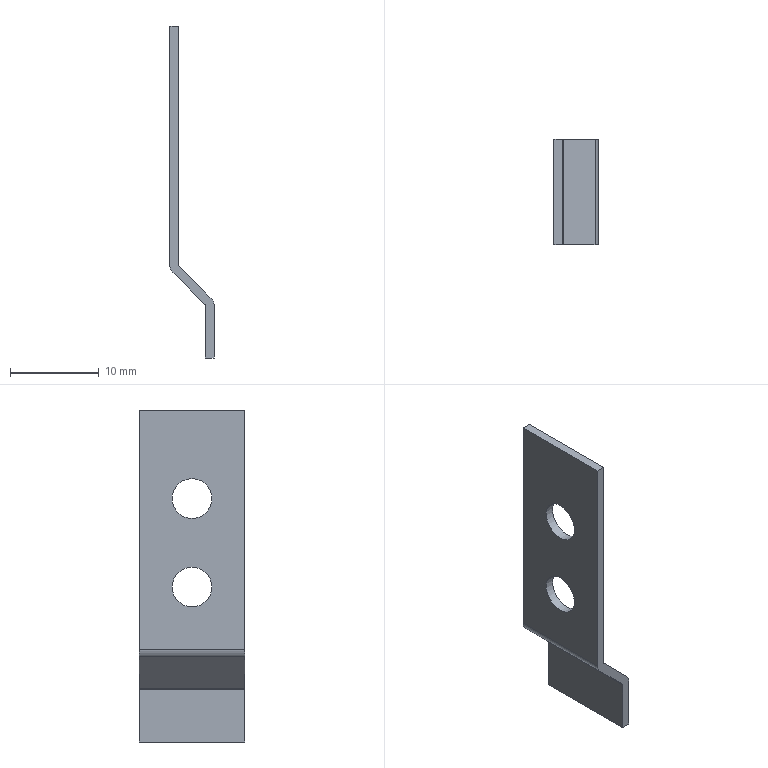Part | STEP file | 1 solid | 16 faces | box 5 x 11.9 x 37.5 mm | volume 433.441 mm3 | plane 10 | cylinder 6 | commonest cylinder face diameters 0.4 x2 2.4 x2 4.5 x2
STEP:
#1=CARTESIAN_POINT('',(0.,0.,0.));
#2=DIRECTION('',(0.,0.,1.));
#3=DIRECTION('',(1.,0.,0.));
#4=AXIS2_PLACEMENT_3D('',#1,#2,#3);
#5=CARTESIAN_POINT('',(0.,0.,-17.75));
#6=VERTEX_POINT('',#5);
#7=CARTESIAN_POINT('',(0.,0.,-20.));
#8=DIRECTION('',(1.,0.,0.));
#9=DIRECTION('',(0.,0.,1.));
#10=AXIS2_PLACEMENT_3D('',#7,#8,#9);
#11=CIRCLE('',#10,2.25);
#12=CARTESIAN_POINT('',(0.,5.95,0.));
#13=DIRECTION('',(-1.,0.,0.));
#14=DIRECTION('',(0.,0.,1.));
#15=AXIS2_PLACEMENT_3D('',#12,#13,#14);
#16=PLANE('',#15);
#17=CARTESIAN_POINT('',(-17.75,-5.95));
#18=CARTESIAN_POINT('',(-17.75,-9.847));
#19=CARTESIAN_POINT('',(-21.125,-7.899));
#20=CARTESIAN_POINT('',(-24.5,-5.95));
#21=CARTESIAN_POINT('',(-21.125,-4.001));
#22=CARTESIAN_POINT('',(-17.75,-2.053));
#23=CARTESIAN_POINT('',(-17.75,-5.95));
#24=(BOUNDED_CURVE()B_SPLINE_CURVE(2,(#17,#18,#19,#20,#21,#22,#23),.UNSPECIFIED.,.T.,.F.)B_SPLINE_CURVE_WITH_KNOTS((1,2,2,2,2,1),(-2.094,0.,2.094,4.189,6.283,8.378),.UNSPECIFIED.)CURVE()GEOMETRIC_REPRESENTATION_ITEM()RATIONAL_B_SPLINE_CURVE((1.,0.5,1.,0.5,1.,0.5,1.))REPRESENTATION_ITEM(''));
#25=(GEOMETRIC_REPRESENTATION_CONTEXT(2)PARAMETRIC_REPRESENTATION_CONTEXT()REPRESENTATION_CONTEXT('',''));
#26=DEFINITIONAL_REPRESENTATION('',(#24),#25);
#27=PCURVE('',#16,#26);
#28=CARTESIAN_POINT('',(0.,0.,-20.));
#29=DIRECTION('',(-1.,0.,0.));
#30=DIRECTION('',(0.,0.,1.));
#31=AXIS2_PLACEMENT_3D('',#28,#29,#30);
#32=CYLINDRICAL_SURFACE('',#31,2.25);
#33=CARTESIAN_POINT('',(6.283,0.));
#34=DIRECTION('',(-1.,0.));
#35=VECTOR('',#34,1.);
#36=LINE('',#33,#35);
#37=(GEOMETRIC_REPRESENTATION_CONTEXT(2)PARAMETRIC_REPRESENTATION_CONTEXT()REPRESENTATION_CONTEXT('',''));
#38=DEFINITIONAL_REPRESENTATION('',(#36),#37);
#39=PCURVE('',#32,#38);
#40=SURFACE_CURVE('',#11,(#27,#39),.PCURVE_S1.);
#41=EDGE_CURVE('',#6,#6,#40,.T.);
#42=ORIENTED_EDGE('',*,*,#41,.T.);
#43=EDGE_LOOP('',(#42));
#44=FACE_BOUND('',#43,.T.);
#45=CARTESIAN_POINT('',(0.,0.,-7.75));
#46=VERTEX_POINT('',#45);
#47=CARTESIAN_POINT('',(0.,0.,-10.));
#48=DIRECTION('',(1.,0.,0.));
#49=DIRECTION('',(0.,0.,1.));
#50=AXIS2_PLACEMENT_3D('',#47,#48,#49);
#51=CIRCLE('',#50,2.25);
#52=CARTESIAN_POINT('',(-7.75,-5.95));
#53=CARTESIAN_POINT('',(-7.75,-9.847));
#54=CARTESIAN_POINT('',(-11.125,-7.899));
#55=CARTESIAN_POINT('',(-14.5,-5.95));
#56=CARTESIAN_POINT('',(-11.125,-4.001));
#57=CARTESIAN_POINT('',(-7.75,-2.053));
#58=CARTESIAN_POINT('',(-7.75,-5.95));
#59=(BOUNDED_CURVE()B_SPLINE_CURVE(2,(#52,#53,#54,#55,#56,#57,#58),.UNSPECIFIED.,.T.,.F.)B_SPLINE_CURVE_WITH_KNOTS((1,2,2,2,2,1),(-2.094,0.,2.094,4.189,6.283,8.378),.UNSPECIFIED.)CURVE()GEOMETRIC_REPRESENTATION_ITEM()RATIONAL_B_SPLINE_CURVE((1.,0.5,1.,0.5,1.,0.5,1.))REPRESENTATION_ITEM(''));
#60=(GEOMETRIC_REPRESENTATION_CONTEXT(2)PARAMETRIC_REPRESENTATION_CONTEXT()REPRESENTATION_CONTEXT('',''));
#61=DEFINITIONAL_REPRESENTATION('',(#59),#60);
#62=PCURVE('',#16,#61);
#63=CARTESIAN_POINT('',(0.,0.,-10.));
#64=DIRECTION('',(-1.,0.,0.));
#65=DIRECTION('',(0.,0.,1.));
#66=AXIS2_PLACEMENT_3D('',#63,#64,#65);
#67=CYLINDRICAL_SURFACE('',#66,2.25);
#68=CARTESIAN_POINT('',(6.283,0.));
#69=DIRECTION('',(-1.,0.));
#70=VECTOR('',#69,1.);
#71=LINE('',#68,#70);
#72=(GEOMETRIC_REPRESENTATION_CONTEXT(2)PARAMETRIC_REPRESENTATION_CONTEXT()REPRESENTATION_CONTEXT('',''));
#73=DEFINITIONAL_REPRESENTATION('',(#71),#72);
#74=PCURVE('',#67,#73);
#75=SURFACE_CURVE('',#51,(#62,#74),.PCURVE_S1.);
#76=EDGE_CURVE('',#46,#46,#75,.T.);
#77=ORIENTED_EDGE('',*,*,#76,.T.);
#78=EDGE_LOOP('',(#77));
#79=FACE_BOUND('',#78,.T.);
#80=CARTESIAN_POINT('',(0.,5.95,0.));
#81=VERTEX_POINT('',#80);
#82=CARTESIAN_POINT('',(0.,5.95,-27.003));
#83=VERTEX_POINT('',#82);
#84=CARTESIAN_POINT('',(0.,5.95,0.));
#85=DIRECTION('',(0.,0.,-1.));
#86=VECTOR('',#85,1.);
#87=LINE('',#84,#86);
#88=CARTESIAN_POINT('',(0.,0.));
#89=DIRECTION('',(-1.,0.));
#90=VECTOR('',#89,1.);
#91=LINE('',#88,#90);
#92=(GEOMETRIC_REPRESENTATION_CONTEXT(2)PARAMETRIC_REPRESENTATION_CONTEXT()REPRESENTATION_CONTEXT('',''));
#93=DEFINITIONAL_REPRESENTATION('',(#91),#92);
#94=PCURVE('',#16,#93);
#95=CARTESIAN_POINT('',(3.8,5.95,-31.583));
#96=DIRECTION('',(0.,-1.,0.));
#97=DIRECTION('',(0.,0.,-1.));
#98=AXIS2_PLACEMENT_3D('',#95,#96,#97);
#99=PLANE('',#98);
#100=CARTESIAN_POINT('',(-31.583,-3.8));
#101=DIRECTION('',(1.,0.));
#102=VECTOR('',#101,1.);
#103=LINE('',#100,#102);
#104=(GEOMETRIC_REPRESENTATION_CONTEXT(2)PARAMETRIC_REPRESENTATION_CONTEXT()REPRESENTATION_CONTEXT('',''));
#105=DEFINITIONAL_REPRESENTATION('',(#103),#104);
#106=PCURVE('',#99,#105);
#107=SURFACE_CURVE('',#87,(#94,#106),.PCURVE_S1.);
#108=EDGE_CURVE('',#81,#83,#107,.T.);
#109=ORIENTED_EDGE('',*,*,#108,.T.);
#110=CARTESIAN_POINT('',(0.,-5.95,-27.003));
#111=VERTEX_POINT('',#110);
#112=CARTESIAN_POINT('',(0.,5.95,-27.003));
#113=DIRECTION('',(0.,-1.,0.));
#114=VECTOR('',#113,1.);
#115=LINE('',#112,#114);
#116=CARTESIAN_POINT('',(-27.003,0.));
#117=DIRECTION('',(0.,-1.));
#118=VECTOR('',#117,1.);
#119=LINE('',#116,#118);
#120=(GEOMETRIC_REPRESENTATION_CONTEXT(2)PARAMETRIC_REPRESENTATION_CONTEXT()REPRESENTATION_CONTEXT('',''));
#121=DEFINITIONAL_REPRESENTATION('',(#119),#120);
#122=PCURVE('',#16,#121);
#123=CARTESIAN_POINT('',(1.2,5.95,-27.003));
#124=DIRECTION('',(0.,-1.,0.));
#125=DIRECTION('',(0.,0.,-1.));
#126=AXIS2_PLACEMENT_3D('',#123,#124,#125);
#127=CYLINDRICAL_SURFACE('',#126,1.2);
#128=CARTESIAN_POINT('',(4.712,0.));
#129=DIRECTION('',(0.,1.));
#130=VECTOR('',#129,1.);
#131=LINE('',#128,#130);
#132=(GEOMETRIC_REPRESENTATION_CONTEXT(2)PARAMETRIC_REPRESENTATION_CONTEXT()REPRESENTATION_CONTEXT('',''));
#133=DEFINITIONAL_REPRESENTATION('',(#131),#132);
#134=PCURVE('',#127,#133);
#135=SURFACE_CURVE('',#115,(#122,#134),.PCURVE_S1.);
#136=EDGE_CURVE('',#83,#111,#135,.T.);
#137=ORIENTED_EDGE('',*,*,#136,.T.);
#138=CARTESIAN_POINT('',(0.,-5.95,0.));
#139=VERTEX_POINT('',#138);
#140=CARTESIAN_POINT('',(0.,-5.95,0.));
#141=DIRECTION('',(0.,0.,1.));
#142=VECTOR('',#141,1.);
#143=LINE('',#140,#142);
#144=CARTESIAN_POINT('',(0.,-11.9));
#145=DIRECTION('',(1.,0.));
#146=VECTOR('',#145,1.);
#147=LINE('',#144,#146);
#148=(GEOMETRIC_REPRESENTATION_CONTEXT(2)PARAMETRIC_REPRESENTATION_CONTEXT()REPRESENTATION_CONTEXT('',''));
#149=DEFINITIONAL_REPRESENTATION('',(#147),#148);
#150=PCURVE('',#16,#149);
#151=CARTESIAN_POINT('',(1.059,-5.95,-27.144));
#152=DIRECTION('',(0.,-1.,0.));
#153=DIRECTION('',(0.,0.,-1.));
#154=AXIS2_PLACEMENT_3D('',#151,#152,#153);
#155=PLANE('',#154);
#156=CARTESIAN_POINT('',(-27.144,-1.059));
#157=DIRECTION('',(-1.,0.));
#158=VECTOR('',#157,1.);
#159=LINE('',#156,#158);
#160=(GEOMETRIC_REPRESENTATION_CONTEXT(2)PARAMETRIC_REPRESENTATION_CONTEXT()REPRESENTATION_CONTEXT('',''));
#161=DEFINITIONAL_REPRESENTATION('',(#159),#160);
#162=PCURVE('',#155,#161);
#163=SURFACE_CURVE('',#143,(#150,#162),.PCURVE_S1.);
#164=EDGE_CURVE('',#111,#139,#163,.T.);
#165=ORIENTED_EDGE('',*,*,#164,.T.);
#166=CARTESIAN_POINT('',(0.,5.95,0.));
#167=DIRECTION('',(0.,1.,0.));
#168=VECTOR('',#167,1.);
#169=LINE('',#166,#168);
#170=CARTESIAN_POINT('',(0.,0.));
#171=DIRECTION('',(0.,1.));
#172=VECTOR('',#171,1.);
#173=LINE('',#170,#172);
#174=(GEOMETRIC_REPRESENTATION_CONTEXT(2)PARAMETRIC_REPRESENTATION_CONTEXT()REPRESENTATION_CONTEXT('',''));
#175=DEFINITIONAL_REPRESENTATION('',(#173),#174);
#176=PCURVE('',#16,#175);
#177=CARTESIAN_POINT('',(1.,5.95,0.));
#178=DIRECTION('',(0.,0.,1.));
#179=DIRECTION('',(1.,0.,0.));
#180=AXIS2_PLACEMENT_3D('',#177,#178,#179);
#181=PLANE('',#180);
#182=CARTESIAN_POINT('',(-1.,0.));
#183=DIRECTION('',(0.,1.));
#184=VECTOR('',#183,1.);
#185=LINE('',#182,#184);
#186=(GEOMETRIC_REPRESENTATION_CONTEXT(2)PARAMETRIC_REPRESENTATION_CONTEXT()REPRESENTATION_CONTEXT('',''));
#187=DEFINITIONAL_REPRESENTATION('',(#185),#186);
#188=PCURVE('',#181,#187);
#189=SURFACE_CURVE('',#169,(#176,#188),.PCURVE_S1.);
#190=EDGE_CURVE('',#139,#81,#189,.T.);
#191=ORIENTED_EDGE('',*,*,#190,.T.);
#192=EDGE_LOOP('',(#109,#137,#165,#191));
#193=FACE_BOUND('',#192,.T.);
#194=ADVANCED_FACE('',(#44,#79,#193),#16,.T.);
#195=ORIENTED_EDGE('',*,*,#41,.T.);
#196=CARTESIAN_POINT('',(1.,0.,-17.75));
#197=VERTEX_POINT('',#196);
#198=CARTESIAN_POINT('',(1.,0.,-17.75));
#199=CARTESIAN_POINT('',(0.,0.,-17.75));
#200=B_SPLINE_CURVE_WITH_KNOTS('',1,(#198,#199),.UNSPECIFIED.,.F.,.F.,(2,2),(-1.,0.),.PIECEWISE_BEZIER_KNOTS.);
#201=CARTESIAN_POINT('',(0.,0.));
#202=DIRECTION('',(0.,1.));
#203=VECTOR('',#202,1.);
#204=LINE('',#201,#203);
#205=(GEOMETRIC_REPRESENTATION_CONTEXT(2)PARAMETRIC_REPRESENTATION_CONTEXT()REPRESENTATION_CONTEXT('',''));
#206=DEFINITIONAL_REPRESENTATION('',(#204),#205);
#207=PCURVE('',#32,#206);
#208=CARTESIAN_POINT('',(6.283,0.));
#209=DIRECTION('',(0.,1.));
#210=VECTOR('',#209,1.);
#211=LINE('',#208,#210);
#212=(GEOMETRIC_REPRESENTATION_CONTEXT(2)PARAMETRIC_REPRESENTATION_CONTEXT()REPRESENTATION_CONTEXT('',''));
#213=DEFINITIONAL_REPRESENTATION('',(#211),#212);
#214=PCURVE('',#32,#213);
#215=SEAM_CURVE('',#200,(#207,#214),.PCURVE_S1.);
#216=EDGE_CURVE('',#197,#6,#215,.T.);
#217=ORIENTED_EDGE('',*,*,#216,.F.);
#218=CARTESIAN_POINT('',(1.,0.,-20.));
#219=DIRECTION('',(-1.,0.,0.));
#220=DIRECTION('',(0.,0.,1.));
#221=AXIS2_PLACEMENT_3D('',#218,#219,#220);
#222=CIRCLE('',#221,2.25);
#223=CARTESIAN_POINT('',(0.,-1.));
#224=DIRECTION('',(1.,0.));
#225=VECTOR('',#224,1.);
#226=LINE('',#223,#225);
#227=(GEOMETRIC_REPRESENTATION_CONTEXT(2)PARAMETRIC_REPRESENTATION_CONTEXT()REPRESENTATION_CONTEXT('',''));
#228=DEFINITIONAL_REPRESENTATION('',(#226),#227);
#229=PCURVE('',#32,#228);
#230=CARTESIAN_POINT('',(1.,5.95,0.));
#231=DIRECTION('',(-1.,0.,0.));
#232=DIRECTION('',(0.,0.,1.));
#233=AXIS2_PLACEMENT_3D('',#230,#231,#232);
#234=PLANE('',#233);
#235=CARTESIAN_POINT('',(-20.,-5.95));
#236=DIRECTION('',(1.,0.));
#237=AXIS2_PLACEMENT_2D('',#235,#236);
#238=CIRCLE('',#237,2.25);
#239=(GEOMETRIC_REPRESENTATION_CONTEXT(2)PARAMETRIC_REPRESENTATION_CONTEXT()REPRESENTATION_CONTEXT('',''));
#240=DEFINITIONAL_REPRESENTATION('',(#238),#239);
#241=PCURVE('',#234,#240);
#242=SURFACE_CURVE('',#222,(#229,#241),.PCURVE_S1.);
#243=EDGE_CURVE('',#197,#197,#242,.T.);
#244=ORIENTED_EDGE('',*,*,#243,.T.);
#245=ORIENTED_EDGE('',*,*,#216,.T.);
#246=EDGE_LOOP('',(#195,#217,#244,#245));
#247=FACE_BOUND('',#246,.F.);
#248=ADVANCED_FACE('',(#247),#32,.F.);
#249=ORIENTED_EDGE('',*,*,#76,.T.);
#250=CARTESIAN_POINT('',(1.,0.,-7.75));
#251=VERTEX_POINT('',#250);
#252=CARTESIAN_POINT('',(1.,0.,-7.75));
#253=CARTESIAN_POINT('',(0.,0.,-7.75));
#254=B_SPLINE_CURVE_WITH_KNOTS('',1,(#252,#253),.UNSPECIFIED.,.F.,.F.,(2,2),(-1.,0.),.PIECEWISE_BEZIER_KNOTS.);
#255=CARTESIAN_POINT('',(0.,0.));
#256=DIRECTION('',(0.,1.));
#257=VECTOR('',#256,1.);
#258=LINE('',#255,#257);
#259=(GEOMETRIC_REPRESENTATION_CONTEXT(2)PARAMETRIC_REPRESENTATION_CONTEXT()REPRESENTATION_CONTEXT('',''));
#260=DEFINITIONAL_REPRESENTATION('',(#258),#259);
#261=PCURVE('',#67,#260);
#262=CARTESIAN_POINT('',(6.283,0.));
#263=DIRECTION('',(0.,1.));
#264=VECTOR('',#263,1.);
#265=LINE('',#262,#264);
#266=(GEOMETRIC_REPRESENTATION_CONTEXT(2)PARAMETRIC_REPRESENTATION_CONTEXT()REPRESENTATION_CONTEXT('',''));
#267=DEFINITIONAL_REPRESENTATION('',(#265),#266);
#268=PCURVE('',#67,#267);
#269=SEAM_CURVE('',#254,(#261,#268),.PCURVE_S1.);
#270=EDGE_CURVE('',#251,#46,#269,.T.);
#271=ORIENTED_EDGE('',*,*,#270,.F.);
#272=CARTESIAN_POINT('',(1.,0.,-10.));
#273=DIRECTION('',(-1.,0.,0.));
#274=DIRECTION('',(0.,0.,1.));
#275=AXIS2_PLACEMENT_3D('',#272,#273,#274);
#276=CIRCLE('',#275,2.25);
#277=CARTESIAN_POINT('',(0.,-1.));
#278=DIRECTION('',(1.,0.));
#279=VECTOR('',#278,1.);
#280=LINE('',#277,#279);
#281=(GEOMETRIC_REPRESENTATION_CONTEXT(2)PARAMETRIC_REPRESENTATION_CONTEXT()REPRESENTATION_CONTEXT('',''));
#282=DEFINITIONAL_REPRESENTATION('',(#280),#281);
#283=PCURVE('',#67,#282);
#284=CARTESIAN_POINT('',(-10.,-5.95));
#285=DIRECTION('',(1.,0.));
#286=AXIS2_PLACEMENT_2D('',#284,#285);
#287=CIRCLE('',#286,2.25);
#288=(GEOMETRIC_REPRESENTATION_CONTEXT(2)PARAMETRIC_REPRESENTATION_CONTEXT()REPRESENTATION_CONTEXT('',''));
#289=DEFINITIONAL_REPRESENTATION('',(#287),#288);
#290=PCURVE('',#234,#289);
#291=SURFACE_CURVE('',#276,(#283,#290),.PCURVE_S1.);
#292=EDGE_CURVE('',#251,#251,#291,.T.);
#293=ORIENTED_EDGE('',*,*,#292,.T.);
#294=ORIENTED_EDGE('',*,*,#270,.T.);
#295=EDGE_LOOP('',(#249,#271,#293,#294));
#296=FACE_BOUND('',#295,.F.);
#297=ADVANCED_FACE('',(#296),#67,.F.);
#298=CARTESIAN_POINT('',(0.3515,5.95,-27.851));
#299=VERTEX_POINT('',#298);
#300=CARTESIAN_POINT('',(1.2,5.95,-27.003));
#301=DIRECTION('',(0.,-1.,0.));
#302=DIRECTION('',(0.,0.,-1.));
#303=AXIS2_PLACEMENT_3D('',#300,#301,#302);
#304=CIRCLE('',#303,1.2);
#305=CARTESIAN_POINT('',(0.,0.));
#306=DIRECTION('',(1.,0.));
#307=VECTOR('',#306,1.);
#308=LINE('',#305,#307);
#309=(GEOMETRIC_REPRESENTATION_CONTEXT(2)PARAMETRIC_REPRESENTATION_CONTEXT()REPRESENTATION_CONTEXT('',''));
#310=DEFINITIONAL_REPRESENTATION('',(#308),#309);
#311=PCURVE('',#127,#310);
#312=CARTESIAN_POINT('',(-4.58,-2.6));
#313=DIRECTION('',(1.,0.));
#314=AXIS2_PLACEMENT_2D('',#312,#313);
#315=CIRCLE('',#314,1.2);
#316=(GEOMETRIC_REPRESENTATION_CONTEXT(2)PARAMETRIC_REPRESENTATION_CONTEXT()REPRESENTATION_CONTEXT('',''));
#317=DEFINITIONAL_REPRESENTATION('',(#315),#316);
#318=PCURVE('',#99,#317);
#319=SURFACE_CURVE('',#304,(#311,#318),.PCURVE_S1.);
#320=EDGE_CURVE('',#83,#299,#319,.T.);
#321=ORIENTED_EDGE('',*,*,#320,.T.);
#322=CARTESIAN_POINT('',(0.3515,-5.95,-27.851));
#323=VERTEX_POINT('',#322);
#324=CARTESIAN_POINT('',(0.3515,5.95,-27.851));
#325=DIRECTION('',(0.,-1.,0.));
#326=VECTOR('',#325,1.);
#327=LINE('',#324,#326);
#328=CARTESIAN_POINT('',(5.498,0.));
#329=DIRECTION('',(0.,1.));
#330=VECTOR('',#329,1.);
#331=LINE('',#328,#330);
#332=(GEOMETRIC_REPRESENTATION_CONTEXT(2)PARAMETRIC_REPRESENTATION_CONTEXT()REPRESENTATION_CONTEXT('',''));
#333=DEFINITIONAL_REPRESENTATION('',(#331),#332);
#334=PCURVE('',#127,#333);
#335=CARTESIAN_POINT('',(0.,5.95,-27.5));
#336=DIRECTION('',(-0.7071,0.,-0.7071));
#337=DIRECTION('',(-0.7071,0.,0.7071));
#338=AXIS2_PLACEMENT_3D('',#335,#336,#337);
#339=PLANE('',#338);
#340=CARTESIAN_POINT('',(-0.4971,0.));
#341=DIRECTION('',(0.,-1.));
#342=VECTOR('',#341,1.);
#343=LINE('',#340,#342);
#344=(GEOMETRIC_REPRESENTATION_CONTEXT(2)PARAMETRIC_REPRESENTATION_CONTEXT()REPRESENTATION_CONTEXT('',''));
#345=DEFINITIONAL_REPRESENTATION('',(#343),#344);
#346=PCURVE('',#339,#345);
#347=SURFACE_CURVE('',#327,(#334,#346),.PCURVE_S1.);
#348=EDGE_CURVE('',#299,#323,#347,.T.);
#349=ORIENTED_EDGE('',*,*,#348,.T.);
#350=CARTESIAN_POINT('',(1.2,-5.95,-27.003));
#351=DIRECTION('',(0.,1.,0.));
#352=DIRECTION('',(0.,0.,-1.));
#353=AXIS2_PLACEMENT_3D('',#350,#351,#352);
#354=CIRCLE('',#353,1.2);
#355=CARTESIAN_POINT('',(6.283,11.9));
#356=DIRECTION('',(-1.,0.));
#357=VECTOR('',#356,1.);
#358=LINE('',#355,#357);
#359=(GEOMETRIC_REPRESENTATION_CONTEXT(2)PARAMETRIC_REPRESENTATION_CONTEXT()REPRESENTATION_CONTEXT('',''));
#360=DEFINITIONAL_REPRESENTATION('',(#358),#359);
#361=PCURVE('',#127,#360);
#362=CARTESIAN_POINT('',(1.059,0.1414));
#363=CARTESIAN_POINT('',(1.059,-1.937));
#364=CARTESIAN_POINT('',(-0.7414,-0.8978));
#365=CARTESIAN_POINT('',(-2.541,0.1414));
#366=CARTESIAN_POINT('',(-0.7414,1.181));
#367=CARTESIAN_POINT('',(1.059,2.22));
#368=CARTESIAN_POINT('',(1.059,0.1414));
#369=(BOUNDED_CURVE()B_SPLINE_CURVE(2,(#362,#363,#364,#365,#366,#367,#368),.UNSPECIFIED.,.T.,.F.)B_SPLINE_CURVE_WITH_KNOTS((1,2,2,2,2,1),(-2.094,0.,2.094,4.189,6.283,8.378),.UNSPECIFIED.)CURVE()GEOMETRIC_REPRESENTATION_ITEM()RATIONAL_B_SPLINE_CURVE((1.,0.5,1.,0.5,1.,0.5,1.))REPRESENTATION_ITEM(''));
#370=(GEOMETRIC_REPRESENTATION_CONTEXT(2)PARAMETRIC_REPRESENTATION_CONTEXT()REPRESENTATION_CONTEXT('',''));
#371=DEFINITIONAL_REPRESENTATION('',(#369),#370);
#372=PCURVE('',#155,#371);
#373=SURFACE_CURVE('',#354,(#361,#372),.PCURVE_S1.);
#374=EDGE_CURVE('',#323,#111,#373,.T.);
#375=ORIENTED_EDGE('',*,*,#374,.T.);
#376=ORIENTED_EDGE('',*,*,#136,.F.);
#377=EDGE_LOOP('',(#321,#349,#375,#376));
#378=FACE_BOUND('',#377,.T.);
#379=ADVANCED_FACE('',(#378),#127,.T.);
#380=CARTESIAN_POINT('',(1.,5.95,-27.003));
#381=VERTEX_POINT('',#380);
#382=CARTESIAN_POINT('',(1.,5.95,0.));
#383=VERTEX_POINT('',#382);
#384=CARTESIAN_POINT('',(1.,5.95,-31.583));
#385=DIRECTION('',(0.,0.,1.));
#386=VECTOR('',#385,1.);
#387=LINE('',#384,#386);
#388=CARTESIAN_POINT('',(0.,-2.8));
#389=DIRECTION('',(-1.,0.));
#390=VECTOR('',#389,1.);
#391=LINE('',#388,#390);
#392=(GEOMETRIC_REPRESENTATION_CONTEXT(2)PARAMETRIC_REPRESENTATION_CONTEXT()REPRESENTATION_CONTEXT('',''));
#393=DEFINITIONAL_REPRESENTATION('',(#391),#392);
#394=PCURVE('',#99,#393);
#395=CARTESIAN_POINT('',(-31.583,0.));
#396=DIRECTION('',(1.,0.));
#397=VECTOR('',#396,1.);
#398=LINE('',#395,#397);
#399=(GEOMETRIC_REPRESENTATION_CONTEXT(2)PARAMETRIC_REPRESENTATION_CONTEXT()REPRESENTATION_CONTEXT('',''));
#400=DEFINITIONAL_REPRESENTATION('',(#398),#399);
#401=PCURVE('',#234,#400);
#402=SURFACE_CURVE('',#387,(#394,#401),.PCURVE_S1.);
#403=EDGE_CURVE('',#381,#383,#402,.T.);
#404=ORIENTED_EDGE('',*,*,#403,.F.);
#405=CARTESIAN_POINT('',(1.059,5.95,-27.144));
#406=VERTEX_POINT('',#405);
#407=CARTESIAN_POINT('',(1.2,5.95,-27.003));
#408=DIRECTION('',(0.,-1.,0.));
#409=DIRECTION('',(0.,0.,-1.));
#410=AXIS2_PLACEMENT_3D('',#407,#408,#409);
#411=CIRCLE('',#410,0.2);
#412=CARTESIAN_POINT('',(-4.58,-2.6));
#413=DIRECTION('',(1.,0.));
#414=AXIS2_PLACEMENT_2D('',#412,#413);
#415=CIRCLE('',#414,0.2);
#416=(GEOMETRIC_REPRESENTATION_CONTEXT(2)PARAMETRIC_REPRESENTATION_CONTEXT()REPRESENTATION_CONTEXT('',''));
#417=DEFINITIONAL_REPRESENTATION('',(#415),#416);
#418=PCURVE('',#99,#417);
#419=CARTESIAN_POINT('',(1.2,5.95,-27.003));
#420=DIRECTION('',(0.,-1.,0.));
#421=DIRECTION('',(0.,0.,-1.));
#422=AXIS2_PLACEMENT_3D('',#419,#420,#421);
#423=CYLINDRICAL_SURFACE('',#422,0.2);
#424=CARTESIAN_POINT('',(0.,0.));
#425=DIRECTION('',(1.,0.));
#426=VECTOR('',#425,1.);
#427=LINE('',#424,#426);
#428=(GEOMETRIC_REPRESENTATION_CONTEXT(2)PARAMETRIC_REPRESENTATION_CONTEXT()REPRESENTATION_CONTEXT('',''));
#429=DEFINITIONAL_REPRESENTATION('',(#427),#428);
#430=PCURVE('',#423,#429);
#431=SURFACE_CURVE('',#411,(#418,#430),.PCURVE_S1.);
#432=EDGE_CURVE('',#381,#406,#431,.T.);
#433=ORIENTED_EDGE('',*,*,#432,.T.);
#434=CARTESIAN_POINT('',(4.649,5.95,-30.734));
#435=VERTEX_POINT('',#434);
#436=CARTESIAN_POINT('',(1.059,5.95,-27.144));
#437=DIRECTION('',(0.7071,0.,-0.7071));
#438=VECTOR('',#437,1.);
#439=LINE('',#436,#438);
#440=CARTESIAN_POINT('',(-4.438,-2.741));
#441=DIRECTION('',(0.7071,0.7071));
#442=VECTOR('',#441,1.);
#443=LINE('',#440,#442);
#444=(GEOMETRIC_REPRESENTATION_CONTEXT(2)PARAMETRIC_REPRESENTATION_CONTEXT()REPRESENTATION_CONTEXT('',''));
#445=DEFINITIONAL_REPRESENTATION('',(#443),#444);
#446=PCURVE('',#99,#445);
#447=CARTESIAN_POINT('',(0.7071,5.95,-26.793));
#448=DIRECTION('',(-0.7071,0.,-0.7071));
#449=DIRECTION('',(-0.7071,0.,0.7071));
#450=AXIS2_PLACEMENT_3D('',#447,#448,#449);
#451=PLANE('',#450);
#452=CARTESIAN_POINT('',(-0.4971,0.));
#453=DIRECTION('',(-1.,0.));
#454=VECTOR('',#453,1.);
#455=LINE('',#452,#454);
#456=(GEOMETRIC_REPRESENTATION_CONTEXT(2)PARAMETRIC_REPRESENTATION_CONTEXT()REPRESENTATION_CONTEXT('',''));
#457=DEFINITIONAL_REPRESENTATION('',(#455),#456);
#458=PCURVE('',#451,#457);
#459=SURFACE_CURVE('',#439,(#446,#458),.PCURVE_S1.);
#460=EDGE_CURVE('',#406,#435,#459,.T.);
#461=ORIENTED_EDGE('',*,*,#460,.T.);
#462=CARTESIAN_POINT('',(5.,5.95,-31.583));
#463=VERTEX_POINT('',#462);
#464=CARTESIAN_POINT('',(3.8,5.95,-31.583));
#465=DIRECTION('',(0.,1.,0.));
#466=DIRECTION('',(0.,0.,-1.));
#467=AXIS2_PLACEMENT_3D('',#464,#465,#466);
#468=CIRCLE('',#467,1.2);
#469=CARTESIAN_POINT('',(1.2,0.));
#470=CARTESIAN_POINT('',(1.2,-2.078));
#471=CARTESIAN_POINT('',(-0.6,-1.039));
#472=CARTESIAN_POINT('',(-2.4,0.));
#473=CARTESIAN_POINT('',(-0.6,1.039));
#474=CARTESIAN_POINT('',(1.2,2.078));
#475=CARTESIAN_POINT('',(1.2,0.));
#476=(BOUNDED_CURVE()B_SPLINE_CURVE(2,(#469,#470,#471,#472,#473,#474,#475),.UNSPECIFIED.,.T.,.F.)B_SPLINE_CURVE_WITH_KNOTS((1,2,2,2,2,1),(-2.094,0.,2.094,4.189,6.283,8.378),.UNSPECIFIED.)CURVE()GEOMETRIC_REPRESENTATION_ITEM()RATIONAL_B_SPLINE_CURVE((1.,0.5,1.,0.5,1.,0.5,1.))REPRESENTATION_ITEM(''));
#477=(GEOMETRIC_REPRESENTATION_CONTEXT(2)PARAMETRIC_REPRESENTATION_CONTEXT()REPRESENTATION_CONTEXT('',''));
#478=DEFINITIONAL_REPRESENTATION('',(#476),#477);
#479=PCURVE('',#99,#478);
#480=CARTESIAN_POINT('',(3.8,5.95,-31.583));
#481=DIRECTION('',(0.,-1.,0.));
#482=DIRECTION('',(0.,0.,-1.));
#483=AXIS2_PLACEMENT_3D('',#480,#481,#482);
#484=CYLINDRICAL_SURFACE('',#483,1.2);
#485=CARTESIAN_POINT('',(6.283,0.));
#486=DIRECTION('',(-1.,0.));
#487=VECTOR('',#486,1.);
#488=LINE('',#485,#487);
#489=(GEOMETRIC_REPRESENTATION_CONTEXT(2)PARAMETRIC_REPRESENTATION_CONTEXT()REPRESENTATION_CONTEXT('',''));
#490=DEFINITIONAL_REPRESENTATION('',(#488),#489);
#491=PCURVE('',#484,#490);
#492=SURFACE_CURVE('',#468,(#479,#491),.PCURVE_S1.);
#493=EDGE_CURVE('',#435,#463,#492,.T.);
#494=ORIENTED_EDGE('',*,*,#493,.T.);
#495=CARTESIAN_POINT('',(5.,5.95,-37.5));
#496=VERTEX_POINT('',#495);
#497=CARTESIAN_POINT('',(5.,5.95,-30.734));
#498=DIRECTION('',(0.,0.,-1.));
#499=VECTOR('',#498,1.);
#500=LINE('',#497,#499);
#501=CARTESIAN_POINT('',(-0.8485,1.2));
#502=DIRECTION('',(1.,0.));
#503=VECTOR('',#502,1.);
#504=LINE('',#501,#503);
#505=(GEOMETRIC_REPRESENTATION_CONTEXT(2)PARAMETRIC_REPRESENTATION_CONTEXT()REPRESENTATION_CONTEXT('',''));
#506=DEFINITIONAL_REPRESENTATION('',(#504),#505);
#507=PCURVE('',#99,#506);
#508=CARTESIAN_POINT('',(5.,5.95,-31.5));
#509=DIRECTION('',(-1.,0.,0.));
#510=DIRECTION('',(0.,0.,1.));
#511=AXIS2_PLACEMENT_3D('',#508,#509,#510);
#512=PLANE('',#511);
#513=CARTESIAN_POINT('',(0.7657,0.));
#514=DIRECTION('',(-1.,0.));
#515=VECTOR('',#514,1.);
#516=LINE('',#513,#515);
#517=(GEOMETRIC_REPRESENTATION_CONTEXT(2)PARAMETRIC_REPRESENTATION_CONTEXT()REPRESENTATION_CONTEXT('',''));
#518=DEFINITIONAL_REPRESENTATION('',(#516),#517);
#519=PCURVE('',#512,#518);
#520=SURFACE_CURVE('',#500,(#507,#519),.PCURVE_S1.);
#521=EDGE_CURVE('',#463,#496,#520,.T.);
#522=ORIENTED_EDGE('',*,*,#521,.T.);
#523=CARTESIAN_POINT('',(4.,5.95,-37.5));
#524=VERTEX_POINT('',#523);
#525=CARTESIAN_POINT('',(4.,5.95,-37.5));
#526=DIRECTION('',(1.,0.,0.));
#527=VECTOR('',#526,1.);
#528=LINE('',#525,#527);
#529=CARTESIAN_POINT('',(5.917,0.2));
#530=DIRECTION('',(0.,1.));
#531=VECTOR('',#530,1.);
#532=LINE('',#529,#531);
#533=(GEOMETRIC_REPRESENTATION_CONTEXT(2)PARAMETRIC_REPRESENTATION_CONTEXT()REPRESENTATION_CONTEXT('',''));
#534=DEFINITIONAL_REPRESENTATION('',(#532),#533);
#535=PCURVE('',#99,#534);
#536=CARTESIAN_POINT('',(4.,5.95,-37.5));
#537=DIRECTION('',(0.,0.,-1.));
#538=DIRECTION('',(-1.,0.,0.));
#539=AXIS2_PLACEMENT_3D('',#536,#537,#538);
#540=PLANE('',#539);
#541=CARTESIAN_POINT('',(0.,0.));
#542=DIRECTION('',(-1.,0.));
#543=VECTOR('',#542,1.);
#544=LINE('',#541,#543);
#545=(GEOMETRIC_REPRESENTATION_CONTEXT(2)PARAMETRIC_REPRESENTATION_CONTEXT()REPRESENTATION_CONTEXT('',''));
#546=DEFINITIONAL_REPRESENTATION('',(#544),#545);
#547=PCURVE('',#540,#546);
#548=SURFACE_CURVE('',#528,(#535,#547),.PCURVE_S1.);
#549=EDGE_CURVE('',#524,#496,#548,.T.);
#550=ORIENTED_EDGE('',*,*,#549,.F.);
#551=CARTESIAN_POINT('',(4.,5.95,-31.583));
#552=VERTEX_POINT('',#551);
#553=CARTESIAN_POINT('',(4.,5.95,-31.5));
#554=DIRECTION('',(0.,0.,-1.));
#555=VECTOR('',#554,1.);
#556=LINE('',#553,#555);
#557=CARTESIAN_POINT('',(-0.08284,0.2));
#558=DIRECTION('',(1.,0.));
#559=VECTOR('',#558,1.);
#560=LINE('',#557,#559);
#561=(GEOMETRIC_REPRESENTATION_CONTEXT(2)PARAMETRIC_REPRESENTATION_CONTEXT()REPRESENTATION_CONTEXT('',''));
#562=DEFINITIONAL_REPRESENTATION('',(#560),#561);
#563=PCURVE('',#99,#562);
#564=CARTESIAN_POINT('',(4.,5.95,-31.5));
#565=DIRECTION('',(-1.,0.,0.));
#566=DIRECTION('',(0.,0.,1.));
#567=AXIS2_PLACEMENT_3D('',#564,#565,#566);
#568=PLANE('',#567);
#569=CARTESIAN_POINT('',(0.,0.));
#570=DIRECTION('',(-1.,0.));
#571=VECTOR('',#570,1.);
#572=LINE('',#569,#571);
#573=(GEOMETRIC_REPRESENTATION_CONTEXT(2)PARAMETRIC_REPRESENTATION_CONTEXT()REPRESENTATION_CONTEXT('',''));
#574=DEFINITIONAL_REPRESENTATION('',(#572),#573);
#575=PCURVE('',#568,#574);
#576=SURFACE_CURVE('',#556,(#563,#575),.PCURVE_S1.);
#577=EDGE_CURVE('',#552,#524,#576,.T.);
#578=ORIENTED_EDGE('',*,*,#577,.F.);
#579=CARTESIAN_POINT('',(3.941,5.95,-31.441));
#580=VERTEX_POINT('',#579);
#581=CARTESIAN_POINT('',(3.8,5.95,-31.583));
#582=DIRECTION('',(0.,-1.,0.));
#583=DIRECTION('',(0.,0.,-1.));
#584=AXIS2_PLACEMENT_3D('',#581,#582,#583);
#585=CIRCLE('',#584,0.2);
#586=CARTESIAN_POINT('',(0.,0.));
#587=DIRECTION('',(1.,0.));
#588=AXIS2_PLACEMENT_2D('',#586,#587);
#589=CIRCLE('',#588,0.2);
#590=(GEOMETRIC_REPRESENTATION_CONTEXT(2)PARAMETRIC_REPRESENTATION_CONTEXT()REPRESENTATION_CONTEXT('',''));
#591=DEFINITIONAL_REPRESENTATION('',(#589),#590);
#592=PCURVE('',#99,#591);
#593=CARTESIAN_POINT('',(3.8,5.95,-31.583));
#594=DIRECTION('',(0.,-1.,0.));
#595=DIRECTION('',(0.,0.,-1.));
#596=AXIS2_PLACEMENT_3D('',#593,#594,#595);
#597=CYLINDRICAL_SURFACE('',#596,0.2);
#598=CARTESIAN_POINT('',(0.,0.));
#599=DIRECTION('',(1.,0.));
#600=VECTOR('',#599,1.);
#601=LINE('',#598,#600);
#602=(GEOMETRIC_REPRESENTATION_CONTEXT(2)PARAMETRIC_REPRESENTATION_CONTEXT()REPRESENTATION_CONTEXT('',''));
#603=DEFINITIONAL_REPRESENTATION('',(#601),#602);
#604=PCURVE('',#597,#603);
#605=SURFACE_CURVE('',#585,(#592,#604),.PCURVE_S1.);
#606=EDGE_CURVE('',#552,#580,#605,.T.);
#607=ORIENTED_EDGE('',*,*,#606,.T.);
#608=CARTESIAN_POINT('',(0.,5.95,-27.5));
#609=DIRECTION('',(0.7071,0.,-0.7071));
#610=VECTOR('',#609,1.);
#611=LINE('',#608,#610);
#612=CARTESIAN_POINT('',(-4.083,-3.8));
#613=DIRECTION('',(0.7071,0.7071));
#614=VECTOR('',#613,1.);
#615=LINE('',#612,#614);
#616=(GEOMETRIC_REPRESENTATION_CONTEXT(2)PARAMETRIC_REPRESENTATION_CONTEXT()REPRESENTATION_CONTEXT('',''));
#617=DEFINITIONAL_REPRESENTATION('',(#615),#616);
#618=PCURVE('',#99,#617);
#619=CARTESIAN_POINT('',(0.,0.));
#620=DIRECTION('',(-1.,0.));
#621=VECTOR('',#620,1.);
#622=LINE('',#619,#621);
#623=(GEOMETRIC_REPRESENTATION_CONTEXT(2)PARAMETRIC_REPRESENTATION_CONTEXT()REPRESENTATION_CONTEXT('',''));
#624=DEFINITIONAL_REPRESENTATION('',(#622),#623);
#625=PCURVE('',#339,#624);
#626=SURFACE_CURVE('',#611,(#618,#625),.PCURVE_S1.);
#627=EDGE_CURVE('',#299,#580,#626,.T.);
#628=ORIENTED_EDGE('',*,*,#627,.F.);
#629=ORIENTED_EDGE('',*,*,#320,.F.);
#630=ORIENTED_EDGE('',*,*,#108,.F.);
#631=CARTESIAN_POINT('',(3.8,5.95,0.));
#632=DIRECTION('',(-1.,0.,0.));
#633=VECTOR('',#632,1.);
#634=LINE('',#631,#633);
#635=CARTESIAN_POINT('',(-31.583,0.));
#636=DIRECTION('',(0.,-1.));
#637=VECTOR('',#636,1.);
#638=LINE('',#635,#637);
#639=(GEOMETRIC_REPRESENTATION_CONTEXT(2)PARAMETRIC_REPRESENTATION_CONTEXT()REPRESENTATION_CONTEXT('',''));
#640=DEFINITIONAL_REPRESENTATION('',(#638),#639);
#641=PCURVE('',#99,#640);
#642=CARTESIAN_POINT('',(2.8,0.));
#643=DIRECTION('',(-1.,0.));
#644=VECTOR('',#643,1.);
#645=LINE('',#642,#644);
#646=(GEOMETRIC_REPRESENTATION_CONTEXT(2)PARAMETRIC_REPRESENTATION_CONTEXT()REPRESENTATION_CONTEXT('',''));
#647=DEFINITIONAL_REPRESENTATION('',(#645),#646);
#648=PCURVE('',#181,#647);
#649=SURFACE_CURVE('',#634,(#641,#648),.PCURVE_S1.);
#650=EDGE_CURVE('',#383,#81,#649,.T.);
#651=ORIENTED_EDGE('',*,*,#650,.F.);
#652=EDGE_LOOP('',(#404,#433,#461,#494,#522,#550,#578,#607,#628,#629,#630,#651));
#653=FACE_BOUND('',#652,.T.);
#654=ADVANCED_FACE('',(#653),#99,.F.);
#655=ORIENTED_EDGE('',*,*,#650,.T.);
#656=ORIENTED_EDGE('',*,*,#190,.F.);
#657=CARTESIAN_POINT('',(1.,-5.95,0.));
#658=VERTEX_POINT('',#657);
#659=CARTESIAN_POINT('',(1.,-5.95,0.));
#660=DIRECTION('',(1.,0.,0.));
#661=VECTOR('',#660,1.);
#662=LINE('',#659,#661);
#663=CARTESIAN_POINT('',(0.,-11.9));
#664=DIRECTION('',(1.,0.));
#665=VECTOR('',#664,1.);
#666=LINE('',#663,#665);
#667=(GEOMETRIC_REPRESENTATION_CONTEXT(2)PARAMETRIC_REPRESENTATION_CONTEXT()REPRESENTATION_CONTEXT('',''));
#668=DEFINITIONAL_REPRESENTATION('',(#666),#667);
#669=PCURVE('',#181,#668);
#670=CARTESIAN_POINT('',(-27.144,-0.05858));
#671=DIRECTION('',(0.,1.));
#672=VECTOR('',#671,1.);
#673=LINE('',#670,#672);
#674=(GEOMETRIC_REPRESENTATION_CONTEXT(2)PARAMETRIC_REPRESENTATION_CONTEXT()REPRESENTATION_CONTEXT('',''));
#675=DEFINITIONAL_REPRESENTATION('',(#673),#674);
#676=PCURVE('',#155,#675);
#677=SURFACE_CURVE('',#662,(#669,#676),.PCURVE_S1.);
#678=EDGE_CURVE('',#139,#658,#677,.T.);
#679=ORIENTED_EDGE('',*,*,#678,.T.);
#680=CARTESIAN_POINT('',(1.,5.95,0.));
#681=DIRECTION('',(0.,1.,0.));
#682=VECTOR('',#681,1.);
#683=LINE('',#680,#682);
#684=CARTESIAN_POINT('',(0.,0.));
#685=DIRECTION('',(0.,1.));
#686=VECTOR('',#685,1.);
#687=LINE('',#684,#686);
#688=(GEOMETRIC_REPRESENTATION_CONTEXT(2)PARAMETRIC_REPRESENTATION_CONTEXT()REPRESENTATION_CONTEXT('',''));
#689=DEFINITIONAL_REPRESENTATION('',(#687),#688);
#690=PCURVE('',#181,#689);
#691=CARTESIAN_POINT('',(0.,0.));
#692=DIRECTION('',(0.,1.));
#693=VECTOR('',#692,1.);
#694=LINE('',#691,#693);
#695=(GEOMETRIC_REPRESENTATION_CONTEXT(2)PARAMETRIC_REPRESENTATION_CONTEXT()REPRESENTATION_CONTEXT('',''));
#696=DEFINITIONAL_REPRESENTATION('',(#694),#695);
#697=PCURVE('',#234,#696);
#698=SURFACE_CURVE('',#683,(#690,#697),.PCURVE_S1.);
#699=EDGE_CURVE('',#658,#383,#698,.T.);
#700=ORIENTED_EDGE('',*,*,#699,.T.);
#701=EDGE_LOOP('',(#655,#656,#679,#700));
#702=FACE_BOUND('',#701,.T.);
#703=ADVANCED_FACE('',(#702),#181,.T.);
#704=CARTESIAN_POINT('',(1.,-5.95,-27.003));
#705=VERTEX_POINT('',#704);
#706=CARTESIAN_POINT('',(1.,-5.95,-27.144));
#707=DIRECTION('',(0.,0.,1.));
#708=VECTOR('',#707,1.);
#709=LINE('',#706,#708);
#710=CARTESIAN_POINT('',(0.,-0.05858));
#711=DIRECTION('',(-1.,0.));
#712=VECTOR('',#711,1.);
#713=LINE('',#710,#712);
#714=(GEOMETRIC_REPRESENTATION_CONTEXT(2)PARAMETRIC_REPRESENTATION_CONTEXT()REPRESENTATION_CONTEXT('',''));
#715=DEFINITIONAL_REPRESENTATION('',(#713),#714);
#716=PCURVE('',#155,#715);
#717=CARTESIAN_POINT('',(-27.144,-11.9));
#718=DIRECTION('',(1.,0.));
#719=VECTOR('',#718,1.);
#720=LINE('',#717,#719);
#721=(GEOMETRIC_REPRESENTATION_CONTEXT(2)PARAMETRIC_REPRESENTATION_CONTEXT()REPRESENTATION_CONTEXT('',''));
#722=DEFINITIONAL_REPRESENTATION('',(#720),#721);
#723=PCURVE('',#234,#722);
#724=SURFACE_CURVE('',#709,(#716,#723),.PCURVE_S1.);
#725=EDGE_CURVE('',#705,#658,#724,.T.);
#726=ORIENTED_EDGE('',*,*,#725,.T.);
#727=ORIENTED_EDGE('',*,*,#678,.F.);
#728=ORIENTED_EDGE('',*,*,#164,.F.);
#729=ORIENTED_EDGE('',*,*,#374,.F.);
#730=CARTESIAN_POINT('',(3.941,-5.95,-31.441));
#731=VERTEX_POINT('',#730);
#732=CARTESIAN_POINT('',(0.,-5.95,-27.5));
#733=DIRECTION('',(-0.7071,0.,0.7071));
#734=VECTOR('',#733,1.);
#735=LINE('',#732,#734);
#736=CARTESIAN_POINT('',(0.3556,-1.059));
#737=DIRECTION('',(-0.7071,-0.7071));
#738=VECTOR('',#737,1.);
#739=LINE('',#736,#738);
#740=(GEOMETRIC_REPRESENTATION_CONTEXT(2)PARAMETRIC_REPRESENTATION_CONTEXT()REPRESENTATION_CONTEXT('',''));
#741=DEFINITIONAL_REPRESENTATION('',(#739),#740);
#742=PCURVE('',#155,#741);
#743=CARTESIAN_POINT('',(0.,-11.9));
#744=DIRECTION('',(1.,0.));
#745=VECTOR('',#744,1.);
#746=LINE('',#743,#745);
#747=(GEOMETRIC_REPRESENTATION_CONTEXT(2)PARAMETRIC_REPRESENTATION_CONTEXT()REPRESENTATION_CONTEXT('',''));
#748=DEFINITIONAL_REPRESENTATION('',(#746),#747);
#749=PCURVE('',#339,#748);
#750=SURFACE_CURVE('',#735,(#742,#749),.PCURVE_S1.);
#751=EDGE_CURVE('',#731,#323,#750,.T.);
#752=ORIENTED_EDGE('',*,*,#751,.F.);
#753=CARTESIAN_POINT('',(4.,-5.95,-31.583));
#754=VERTEX_POINT('',#753);
#755=CARTESIAN_POINT('',(3.8,-5.95,-31.583));
#756=DIRECTION('',(0.,1.,0.));
#757=DIRECTION('',(0.,0.,-1.));
#758=AXIS2_PLACEMENT_3D('',#755,#756,#757);
#759=CIRCLE('',#758,0.2);
#760=CARTESIAN_POINT('',(4.638,2.741));
#761=CARTESIAN_POINT('',(4.638,2.395));
#762=CARTESIAN_POINT('',(4.338,2.568));
#763=CARTESIAN_POINT('',(4.038,2.741));
#764=CARTESIAN_POINT('',(4.338,2.915));
#765=CARTESIAN_POINT('',(4.638,3.088));
#766=CARTESIAN_POINT('',(4.638,2.741));
#767=(BOUNDED_CURVE()B_SPLINE_CURVE(2,(#760,#761,#762,#763,#764,#765,#766),.UNSPECIFIED.,.T.,.F.)B_SPLINE_CURVE_WITH_KNOTS((1,2,2,2,2,1),(-2.094,0.,2.094,4.189,6.283,8.378),.UNSPECIFIED.)CURVE()GEOMETRIC_REPRESENTATION_ITEM()RATIONAL_B_SPLINE_CURVE((1.,0.5,1.,0.5,1.,0.5,1.))REPRESENTATION_ITEM(''));
#768=(GEOMETRIC_REPRESENTATION_CONTEXT(2)PARAMETRIC_REPRESENTATION_CONTEXT()REPRESENTATION_CONTEXT('',''));
#769=DEFINITIONAL_REPRESENTATION('',(#767),#768);
#770=PCURVE('',#155,#769);
#771=CARTESIAN_POINT('',(6.283,11.9));
#772=DIRECTION('',(-1.,0.));
#773=VECTOR('',#772,1.);
#774=LINE('',#771,#773);
#775=(GEOMETRIC_REPRESENTATION_CONTEXT(2)PARAMETRIC_REPRESENTATION_CONTEXT()REPRESENTATION_CONTEXT('',''));
#776=DEFINITIONAL_REPRESENTATION('',(#774),#775);
#777=PCURVE('',#597,#776);
#778=SURFACE_CURVE('',#759,(#770,#777),.PCURVE_S1.);
#779=EDGE_CURVE('',#731,#754,#778,.T.);
#780=ORIENTED_EDGE('',*,*,#779,.T.);
#781=CARTESIAN_POINT('',(4.,-5.95,-37.5));
#782=VERTEX_POINT('',#781);
#783=CARTESIAN_POINT('',(4.,-5.95,-31.5));
#784=DIRECTION('',(0.,0.,1.));
#785=VECTOR('',#784,1.);
#786=LINE('',#783,#785);
#787=CARTESIAN_POINT('',(4.356,2.941));
#788=DIRECTION('',(-1.,0.));
#789=VECTOR('',#788,1.);
#790=LINE('',#787,#789);
#791=(GEOMETRIC_REPRESENTATION_CONTEXT(2)PARAMETRIC_REPRESENTATION_CONTEXT()REPRESENTATION_CONTEXT('',''));
#792=DEFINITIONAL_REPRESENTATION('',(#790),#791);
#793=PCURVE('',#155,#792);
#794=CARTESIAN_POINT('',(0.,-11.9));
#795=DIRECTION('',(1.,0.));
#796=VECTOR('',#795,1.);
#797=LINE('',#794,#796);
#798=(GEOMETRIC_REPRESENTATION_CONTEXT(2)PARAMETRIC_REPRESENTATION_CONTEXT()REPRESENTATION_CONTEXT('',''));
#799=DEFINITIONAL_REPRESENTATION('',(#797),#798);
#800=PCURVE('',#568,#799);
#801=SURFACE_CURVE('',#786,(#793,#800),.PCURVE_S1.);
#802=EDGE_CURVE('',#782,#754,#801,.T.);
#803=ORIENTED_EDGE('',*,*,#802,.F.);
#804=CARTESIAN_POINT('',(5.,-5.95,-37.5));
#805=VERTEX_POINT('',#804);
#806=CARTESIAN_POINT('',(4.,-5.95,-37.5));
#807=DIRECTION('',(-1.,0.,0.));
#808=VECTOR('',#807,1.);
#809=LINE('',#806,#808);
#810=CARTESIAN_POINT('',(10.356,2.941));
#811=DIRECTION('',(0.,-1.));
#812=VECTOR('',#811,1.);
#813=LINE('',#810,#812);
#814=(GEOMETRIC_REPRESENTATION_CONTEXT(2)PARAMETRIC_REPRESENTATION_CONTEXT()REPRESENTATION_CONTEXT('',''));
#815=DEFINITIONAL_REPRESENTATION('',(#813),#814);
#816=PCURVE('',#155,#815);
#817=CARTESIAN_POINT('',(0.,-11.9));
#818=DIRECTION('',(1.,0.));
#819=VECTOR('',#818,1.);
#820=LINE('',#817,#819);
#821=(GEOMETRIC_REPRESENTATION_CONTEXT(2)PARAMETRIC_REPRESENTATION_CONTEXT()REPRESENTATION_CONTEXT('',''));
#822=DEFINITIONAL_REPRESENTATION('',(#820),#821);
#823=PCURVE('',#540,#822);
#824=SURFACE_CURVE('',#809,(#816,#823),.PCURVE_S1.);
#825=EDGE_CURVE('',#805,#782,#824,.T.);
#826=ORIENTED_EDGE('',*,*,#825,.F.);
#827=CARTESIAN_POINT('',(5.,-5.95,-31.583));
#828=VERTEX_POINT('',#827);
#829=CARTESIAN_POINT('',(5.,-5.95,-31.583));
#830=DIRECTION('',(0.,0.,1.));
#831=VECTOR('',#830,1.);
#832=LINE('',#829,#831);
#833=CARTESIAN_POINT('',(4.438,3.941));
#834=DIRECTION('',(-1.,0.));
#835=VECTOR('',#834,1.);
#836=LINE('',#833,#835);
#837=(GEOMETRIC_REPRESENTATION_CONTEXT(2)PARAMETRIC_REPRESENTATION_CONTEXT()REPRESENTATION_CONTEXT('',''));
#838=DEFINITIONAL_REPRESENTATION('',(#836),#837);
#839=PCURVE('',#155,#838);
#840=CARTESIAN_POINT('',(-0.08284,-11.9));
#841=DIRECTION('',(1.,0.));
#842=VECTOR('',#841,1.);
#843=LINE('',#840,#842);
#844=(GEOMETRIC_REPRESENTATION_CONTEXT(2)PARAMETRIC_REPRESENTATION_CONTEXT()REPRESENTATION_CONTEXT('',''));
#845=DEFINITIONAL_REPRESENTATION('',(#843),#844);
#846=PCURVE('',#512,#845);
#847=SURFACE_CURVE('',#832,(#839,#846),.PCURVE_S1.);
#848=EDGE_CURVE('',#805,#828,#847,.T.);
#849=ORIENTED_EDGE('',*,*,#848,.T.);
#850=CARTESIAN_POINT('',(4.649,-5.95,-30.734));
#851=VERTEX_POINT('',#850);
#852=CARTESIAN_POINT('',(3.8,-5.95,-31.583));
#853=DIRECTION('',(0.,-1.,0.));
#854=DIRECTION('',(0.,0.,-1.));
#855=AXIS2_PLACEMENT_3D('',#852,#853,#854);
#856=CIRCLE('',#855,1.2);
#857=CARTESIAN_POINT('',(4.438,2.741));
#858=DIRECTION('',(1.,0.));
#859=AXIS2_PLACEMENT_2D('',#857,#858);
#860=CIRCLE('',#859,1.2);
#861=(GEOMETRIC_REPRESENTATION_CONTEXT(2)PARAMETRIC_REPRESENTATION_CONTEXT()REPRESENTATION_CONTEXT('',''));
#862=DEFINITIONAL_REPRESENTATION('',(#860),#861);
#863=PCURVE('',#155,#862);
#864=CARTESIAN_POINT('',(0.,11.9));
#865=DIRECTION('',(1.,0.));
#866=VECTOR('',#865,1.);
#867=LINE('',#864,#866);
#868=(GEOMETRIC_REPRESENTATION_CONTEXT(2)PARAMETRIC_REPRESENTATION_CONTEXT()REPRESENTATION_CONTEXT('',''));
#869=DEFINITIONAL_REPRESENTATION('',(#867),#868);
#870=PCURVE('',#484,#869);
#871=SURFACE_CURVE('',#856,(#863,#870),.PCURVE_S1.);
#872=EDGE_CURVE('',#828,#851,#871,.T.);
#873=ORIENTED_EDGE('',*,*,#872,.T.);
#874=CARTESIAN_POINT('',(1.059,-5.95,-27.144));
#875=VERTEX_POINT('',#874);
#876=CARTESIAN_POINT('',(4.649,-5.95,-30.734));
#877=DIRECTION('',(-0.7071,0.,0.7071));
#878=VECTOR('',#877,1.);
#879=LINE('',#876,#878);
#880=CARTESIAN_POINT('',(3.59,3.59));
#881=DIRECTION('',(-0.7071,-0.7071));
#882=VECTOR('',#881,1.);
#883=LINE('',#880,#882);
#884=(GEOMETRIC_REPRESENTATION_CONTEXT(2)PARAMETRIC_REPRESENTATION_CONTEXT()REPRESENTATION_CONTEXT('',''));
#885=DEFINITIONAL_REPRESENTATION('',(#883),#884);
#886=PCURVE('',#155,#885);
#887=CARTESIAN_POINT('',(-5.574,-11.9));
#888=DIRECTION('',(1.,0.));
#889=VECTOR('',#888,1.);
#890=LINE('',#887,#889);
#891=(GEOMETRIC_REPRESENTATION_CONTEXT(2)PARAMETRIC_REPRESENTATION_CONTEXT()REPRESENTATION_CONTEXT('',''));
#892=DEFINITIONAL_REPRESENTATION('',(#890),#891);
#893=PCURVE('',#451,#892);
#894=SURFACE_CURVE('',#879,(#886,#893),.PCURVE_S1.);
#895=EDGE_CURVE('',#851,#875,#894,.T.);
#896=ORIENTED_EDGE('',*,*,#895,.T.);
#897=CARTESIAN_POINT('',(1.2,-5.95,-27.003));
#898=DIRECTION('',(0.,1.,0.));
#899=DIRECTION('',(0.,0.,-1.));
#900=AXIS2_PLACEMENT_3D('',#897,#898,#899);
#901=CIRCLE('',#900,0.2);
#902=CARTESIAN_POINT('',(0.05858,0.1414));
#903=CARTESIAN_POINT('',(0.05858,-0.205));
#904=CARTESIAN_POINT('',(-0.2414,-0.03178));
#905=CARTESIAN_POINT('',(-0.5414,0.1414));
#906=CARTESIAN_POINT('',(-0.2414,0.3146));
#907=CARTESIAN_POINT('',(0.05858,0.4878));
#908=CARTESIAN_POINT('',(0.05858,0.1414));
#909=(BOUNDED_CURVE()B_SPLINE_CURVE(2,(#902,#903,#904,#905,#906,#907,#908),.UNSPECIFIED.,.T.,.F.)B_SPLINE_CURVE_WITH_KNOTS((1,2,2,2,2,1),(-2.094,0.,2.094,4.189,6.283,8.378),.UNSPECIFIED.)CURVE()GEOMETRIC_REPRESENTATION_ITEM()RATIONAL_B_SPLINE_CURVE((1.,0.5,1.,0.5,1.,0.5,1.))REPRESENTATION_ITEM(''));
#910=(GEOMETRIC_REPRESENTATION_CONTEXT(2)PARAMETRIC_REPRESENTATION_CONTEXT()REPRESENTATION_CONTEXT('',''));
#911=DEFINITIONAL_REPRESENTATION('',(#909),#910);
#912=PCURVE('',#155,#911);
#913=CARTESIAN_POINT('',(6.283,11.9));
#914=DIRECTION('',(-1.,0.));
#915=VECTOR('',#914,1.);
#916=LINE('',#913,#915);
#917=(GEOMETRIC_REPRESENTATION_CONTEXT(2)PARAMETRIC_REPRESENTATION_CONTEXT()REPRESENTATION_CONTEXT('',''));
#918=DEFINITIONAL_REPRESENTATION('',(#916),#917);
#919=PCURVE('',#423,#918);
#920=SURFACE_CURVE('',#901,(#912,#919),.PCURVE_S1.);
#921=EDGE_CURVE('',#875,#705,#920,.T.);
#922=ORIENTED_EDGE('',*,*,#921,.T.);
#923=EDGE_LOOP('',(#726,#727,#728,#729,#752,#780,#803,#826,#849,#873,#896,#922));
#924=FACE_BOUND('',#923,.T.);
#925=ADVANCED_FACE('',(#924),#155,.T.);
#926=ORIENTED_EDGE('',*,*,#243,.T.);
#927=EDGE_LOOP('',(#926));
#928=FACE_BOUND('',#927,.T.);
#929=ORIENTED_EDGE('',*,*,#292,.T.);
#930=EDGE_LOOP('',(#929));
#931=FACE_BOUND('',#930,.T.);
#932=CARTESIAN_POINT('',(1.,5.95,-27.003));
#933=DIRECTION('',(0.,-1.,0.));
#934=VECTOR('',#933,1.);
#935=LINE('',#932,#934);
#936=CARTESIAN_POINT('',(-27.003,0.));
#937=DIRECTION('',(0.,-1.));
#938=VECTOR('',#937,1.);
#939=LINE('',#936,#938);
#940=(GEOMETRIC_REPRESENTATION_CONTEXT(2)PARAMETRIC_REPRESENTATION_CONTEXT()REPRESENTATION_CONTEXT('',''));
#941=DEFINITIONAL_REPRESENTATION('',(#939),#940);
#942=PCURVE('',#234,#941);
#943=CARTESIAN_POINT('',(4.712,0.));
#944=DIRECTION('',(0.,1.));
#945=VECTOR('',#944,1.);
#946=LINE('',#943,#945);
#947=(GEOMETRIC_REPRESENTATION_CONTEXT(2)PARAMETRIC_REPRESENTATION_CONTEXT()REPRESENTATION_CONTEXT('',''));
#948=DEFINITIONAL_REPRESENTATION('',(#946),#947);
#949=PCURVE('',#423,#948);
#950=SURFACE_CURVE('',#935,(#942,#949),.PCURVE_S1.);
#951=EDGE_CURVE('',#381,#705,#950,.T.);
#952=ORIENTED_EDGE('',*,*,#951,.F.);
#953=ORIENTED_EDGE('',*,*,#403,.T.);
#954=ORIENTED_EDGE('',*,*,#699,.F.);
#955=ORIENTED_EDGE('',*,*,#725,.F.);
#956=EDGE_LOOP('',(#952,#953,#954,#955));
#957=FACE_BOUND('',#956,.T.);
#958=ADVANCED_FACE('',(#928,#931,#957),#234,.F.);
#959=ORIENTED_EDGE('',*,*,#627,.T.);
#960=CARTESIAN_POINT('',(3.941,5.95,-31.441));
#961=DIRECTION('',(0.,-1.,0.));
#962=VECTOR('',#961,1.);
#963=LINE('',#960,#962);
#964=CARTESIAN_POINT('',(-5.574,0.));
#965=DIRECTION('',(0.,-1.));
#966=VECTOR('',#965,1.);
#967=LINE('',#964,#966);
#968=(GEOMETRIC_REPRESENTATION_CONTEXT(2)PARAMETRIC_REPRESENTATION_CONTEXT()REPRESENTATION_CONTEXT('',''));
#969=DEFINITIONAL_REPRESENTATION('',(#967),#968);
#970=PCURVE('',#339,#969);
#971=CARTESIAN_POINT('',(2.356,0.));
#972=DIRECTION('',(0.,1.));
#973=VECTOR('',#972,1.);
#974=LINE('',#971,#973);
#975=(GEOMETRIC_REPRESENTATION_CONTEXT(2)PARAMETRIC_REPRESENTATION_CONTEXT()REPRESENTATION_CONTEXT('',''));
#976=DEFINITIONAL_REPRESENTATION('',(#974),#975);
#977=PCURVE('',#597,#976);
#978=SURFACE_CURVE('',#963,(#970,#977),.PCURVE_S1.);
#979=EDGE_CURVE('',#580,#731,#978,.T.);
#980=ORIENTED_EDGE('',*,*,#979,.T.);
#981=ORIENTED_EDGE('',*,*,#751,.T.);
#982=ORIENTED_EDGE('',*,*,#348,.F.);
#983=EDGE_LOOP('',(#959,#980,#981,#982));
#984=FACE_BOUND('',#983,.T.);
#985=ADVANCED_FACE('',(#984),#339,.T.);
#986=ORIENTED_EDGE('',*,*,#921,.T.);
#987=ORIENTED_EDGE('',*,*,#951,.F.);
#988=ORIENTED_EDGE('',*,*,#432,.T.);
#989=CARTESIAN_POINT('',(1.059,5.95,-27.144));
#990=DIRECTION('',(0.,-1.,0.));
#991=VECTOR('',#990,1.);
#992=LINE('',#989,#991);
#993=CARTESIAN_POINT('',(5.498,0.));
#994=DIRECTION('',(0.,1.));
#995=VECTOR('',#994,1.);
#996=LINE('',#993,#995);
#997=(GEOMETRIC_REPRESENTATION_CONTEXT(2)PARAMETRIC_REPRESENTATION_CONTEXT()REPRESENTATION_CONTEXT('',''));
#998=DEFINITIONAL_REPRESENTATION('',(#996),#997);
#999=PCURVE('',#423,#998);
#1000=CARTESIAN_POINT('',(-0.4971,0.));
#1001=DIRECTION('',(0.,-1.));
#1002=VECTOR('',#1001,1.);
#1003=LINE('',#1000,#1002);
#1004=(GEOMETRIC_REPRESENTATION_CONTEXT(2)PARAMETRIC_REPRESENTATION_CONTEXT()REPRESENTATION_CONTEXT('',''));
#1005=DEFINITIONAL_REPRESENTATION('',(#1003),#1004);
#1006=PCURVE('',#451,#1005);
#1007=SURFACE_CURVE('',#992,(#999,#1006),.PCURVE_S1.);
#1008=EDGE_CURVE('',#406,#875,#1007,.T.);
#1009=ORIENTED_EDGE('',*,*,#1008,.T.);
#1010=EDGE_LOOP('',(#986,#987,#988,#1009));
#1011=FACE_BOUND('',#1010,.F.);
#1012=ADVANCED_FACE('',(#1011),#423,.F.);
#1013=ORIENTED_EDGE('',*,*,#779,.T.);
#1014=CARTESIAN_POINT('',(4.,5.95,-31.583));
#1015=DIRECTION('',(0.,1.,0.));
#1016=VECTOR('',#1015,1.);
#1017=LINE('',#1014,#1016);
#1018=CARTESIAN_POINT('',(1.571,0.));
#1019=DIRECTION('',(0.,-1.));
#1020=VECTOR('',#1019,1.);
#1021=LINE('',#1018,#1020);
#1022=(GEOMETRIC_REPRESENTATION_CONTEXT(2)PARAMETRIC_REPRESENTATION_CONTEXT()REPRESENTATION_CONTEXT('',''));
#1023=DEFINITIONAL_REPRESENTATION('',(#1021),#1022);
#1024=PCURVE('',#597,#1023);
#1025=CARTESIAN_POINT('',(-0.08284,0.));
#1026=DIRECTION('',(0.,1.));
#1027=VECTOR('',#1026,1.);
#1028=LINE('',#1025,#1027);
#1029=(GEOMETRIC_REPRESENTATION_CONTEXT(2)PARAMETRIC_REPRESENTATION_CONTEXT()REPRESENTATION_CONTEXT('',''));
#1030=DEFINITIONAL_REPRESENTATION('',(#1028),#1029);
#1031=PCURVE('',#568,#1030);
#1032=SURFACE_CURVE('',#1017,(#1024,#1031),.PCURVE_S1.);
#1033=EDGE_CURVE('',#754,#552,#1032,.T.);
#1034=ORIENTED_EDGE('',*,*,#1033,.T.);
#1035=ORIENTED_EDGE('',*,*,#606,.T.);
#1036=ORIENTED_EDGE('',*,*,#979,.T.);
#1037=EDGE_LOOP('',(#1013,#1034,#1035,#1036));
#1038=FACE_BOUND('',#1037,.F.);
#1039=ADVANCED_FACE('',(#1038),#597,.F.);
#1040=CARTESIAN_POINT('',(4.649,5.95,-30.734));
#1041=DIRECTION('',(0.,-1.,0.));
#1042=VECTOR('',#1041,1.);
#1043=LINE('',#1040,#1042);
#1044=CARTESIAN_POINT('',(-5.574,0.));
#1045=DIRECTION('',(0.,-1.));
#1046=VECTOR('',#1045,1.);
#1047=LINE('',#1044,#1046);
#1048=(GEOMETRIC_REPRESENTATION_CONTEXT(2)PARAMETRIC_REPRESENTATION_CONTEXT()REPRESENTATION_CONTEXT('',''));
#1049=DEFINITIONAL_REPRESENTATION('',(#1047),#1048);
#1050=PCURVE('',#451,#1049);
#1051=CARTESIAN_POINT('',(2.356,0.));
#1052=DIRECTION('',(0.,1.));
#1053=VECTOR('',#1052,1.);
#1054=LINE('',#1051,#1053);
#1055=(GEOMETRIC_REPRESENTATION_CONTEXT(2)PARAMETRIC_REPRESENTATION_CONTEXT()REPRESENTATION_CONTEXT('',''));
#1056=DEFINITIONAL_REPRESENTATION('',(#1054),#1055);
#1057=PCURVE('',#484,#1056);
#1058=SURFACE_CURVE('',#1043,(#1050,#1057),.PCURVE_S1.);
#1059=EDGE_CURVE('',#435,#851,#1058,.T.);
#1060=ORIENTED_EDGE('',*,*,#1059,.F.);
#1061=ORIENTED_EDGE('',*,*,#460,.F.);
#1062=ORIENTED_EDGE('',*,*,#1008,.T.);
#1063=ORIENTED_EDGE('',*,*,#895,.F.);
#1064=EDGE_LOOP('',(#1060,#1061,#1062,#1063));
#1065=FACE_BOUND('',#1064,.T.);
#1066=ADVANCED_FACE('',(#1065),#451,.F.);
#1067=ORIENTED_EDGE('',*,*,#577,.T.);
#1068=CARTESIAN_POINT('',(4.,5.95,-37.5));
#1069=DIRECTION('',(0.,-1.,0.));
#1070=VECTOR('',#1069,1.);
#1071=LINE('',#1068,#1070);
#1072=CARTESIAN_POINT('',(-6.,0.));
#1073=DIRECTION('',(0.,-1.));
#1074=VECTOR('',#1073,1.);
#1075=LINE('',#1072,#1074);
#1076=(GEOMETRIC_REPRESENTATION_CONTEXT(2)PARAMETRIC_REPRESENTATION_CONTEXT()REPRESENTATION_CONTEXT('',''));
#1077=DEFINITIONAL_REPRESENTATION('',(#1075),#1076);
#1078=PCURVE('',#568,#1077);
#1079=CARTESIAN_POINT('',(0.,0.));
#1080=DIRECTION('',(0.,-1.));
#1081=VECTOR('',#1080,1.);
#1082=LINE('',#1079,#1081);
#1083=(GEOMETRIC_REPRESENTATION_CONTEXT(2)PARAMETRIC_REPRESENTATION_CONTEXT()REPRESENTATION_CONTEXT('',''));
#1084=DEFINITIONAL_REPRESENTATION('',(#1082),#1083);
#1085=PCURVE('',#540,#1084);
#1086=SURFACE_CURVE('',#1071,(#1078,#1085),.PCURVE_S1.);
#1087=EDGE_CURVE('',#524,#782,#1086,.T.);
#1088=ORIENTED_EDGE('',*,*,#1087,.T.);
#1089=ORIENTED_EDGE('',*,*,#802,.T.);
#1090=ORIENTED_EDGE('',*,*,#1033,.T.);
#1091=EDGE_LOOP('',(#1067,#1088,#1089,#1090));
#1092=FACE_BOUND('',#1091,.T.);
#1093=ADVANCED_FACE('',(#1092),#568,.T.);
#1094=ORIENTED_EDGE('',*,*,#493,.F.);
#1095=ORIENTED_EDGE('',*,*,#1059,.T.);
#1096=ORIENTED_EDGE('',*,*,#872,.F.);
#1097=CARTESIAN_POINT('',(5.,5.95,-31.583));
#1098=DIRECTION('',(0.,1.,0.));
#1099=VECTOR('',#1098,1.);
#1100=LINE('',#1097,#1099);
#1101=CARTESIAN_POINT('',(1.571,0.));
#1102=DIRECTION('',(0.,-1.));
#1103=VECTOR('',#1102,1.);
#1104=LINE('',#1101,#1103);
#1105=(GEOMETRIC_REPRESENTATION_CONTEXT(2)PARAMETRIC_REPRESENTATION_CONTEXT()REPRESENTATION_CONTEXT('',''));
#1106=DEFINITIONAL_REPRESENTATION('',(#1104),#1105);
#1107=PCURVE('',#484,#1106);
#1108=CARTESIAN_POINT('',(-0.08284,0.));
#1109=DIRECTION('',(0.,1.));
#1110=VECTOR('',#1109,1.);
#1111=LINE('',#1108,#1110);
#1112=(GEOMETRIC_REPRESENTATION_CONTEXT(2)PARAMETRIC_REPRESENTATION_CONTEXT()REPRESENTATION_CONTEXT('',''));
#1113=DEFINITIONAL_REPRESENTATION('',(#1111),#1112);
#1114=PCURVE('',#512,#1113);
#1115=SURFACE_CURVE('',#1100,(#1107,#1114),.PCURVE_S1.);
#1116=EDGE_CURVE('',#828,#463,#1115,.T.);
#1117=ORIENTED_EDGE('',*,*,#1116,.T.);
#1118=EDGE_LOOP('',(#1094,#1095,#1096,#1117));
#1119=FACE_BOUND('',#1118,.T.);
#1120=ADVANCED_FACE('',(#1119),#484,.T.);
#1121=ORIENTED_EDGE('',*,*,#549,.T.);
#1122=CARTESIAN_POINT('',(5.,5.95,-37.5));
#1123=DIRECTION('',(0.,-1.,0.));
#1124=VECTOR('',#1123,1.);
#1125=LINE('',#1122,#1124);
#1126=CARTESIAN_POINT('',(-1.,0.));
#1127=DIRECTION('',(0.,-1.));
#1128=VECTOR('',#1127,1.);
#1129=LINE('',#1126,#1128);
#1130=(GEOMETRIC_REPRESENTATION_CONTEXT(2)PARAMETRIC_REPRESENTATION_CONTEXT()REPRESENTATION_CONTEXT('',''));
#1131=DEFINITIONAL_REPRESENTATION('',(#1129),#1130);
#1132=PCURVE('',#540,#1131);
#1133=CARTESIAN_POINT('',(-6.,0.));
#1134=DIRECTION('',(0.,-1.));
#1135=VECTOR('',#1134,1.);
#1136=LINE('',#1133,#1135);
#1137=(GEOMETRIC_REPRESENTATION_CONTEXT(2)PARAMETRIC_REPRESENTATION_CONTEXT()REPRESENTATION_CONTEXT('',''));
#1138=DEFINITIONAL_REPRESENTATION('',(#1136),#1137);
#1139=PCURVE('',#512,#1138);
#1140=SURFACE_CURVE('',#1125,(#1132,#1139),.PCURVE_S1.);
#1141=EDGE_CURVE('',#496,#805,#1140,.T.);
#1142=ORIENTED_EDGE('',*,*,#1141,.T.);
#1143=ORIENTED_EDGE('',*,*,#825,.T.);
#1144=ORIENTED_EDGE('',*,*,#1087,.F.);
#1145=EDGE_LOOP('',(#1121,#1142,#1143,#1144));
#1146=FACE_BOUND('',#1145,.T.);
#1147=ADVANCED_FACE('',(#1146),#540,.T.);
#1148=ORIENTED_EDGE('',*,*,#1141,.F.);
#1149=ORIENTED_EDGE('',*,*,#521,.F.);
#1150=ORIENTED_EDGE('',*,*,#1116,.F.);
#1151=ORIENTED_EDGE('',*,*,#848,.F.);
#1152=EDGE_LOOP('',(#1148,#1149,#1150,#1151));
#1153=FACE_BOUND('',#1152,.T.);
#1154=ADVANCED_FACE('',(#1153),#512,.F.);
#1155=CLOSED_SHELL('',(#194,#248,#297,#379,#654,#703,#925,#958,#985,#1012,#1039,#1066,#1093,#1120,#1147,#1154));
#1156=MANIFOLD_SOLID_BREP('',#1155);
#1157=(LENGTH_UNIT()NAMED_UNIT(*)SI_UNIT(.MILLI.,.METRE.));
#1158=UNCERTAINTY_MEASURE_WITH_UNIT(LENGTH_MEASURE(0.000001),#1157,'','');
#1159=(NAMED_UNIT(*)PLANE_ANGLE_UNIT()SI_UNIT($,.RADIAN.));
#1160=(NAMED_UNIT(*)SI_UNIT($,.STERADIAN.)SOLID_ANGLE_UNIT());
#1161=(GEOMETRIC_REPRESENTATION_CONTEXT(3)GLOBAL_UNCERTAINTY_ASSIGNED_CONTEXT((#1158))GLOBAL_UNIT_ASSIGNED_CONTEXT((#1157,#1159,#1160))REPRESENTATION_CONTEXT('',''));
#1162=ADVANCED_BREP_SHAPE_REPRESENTATION('',(#4,#1156),#1161);